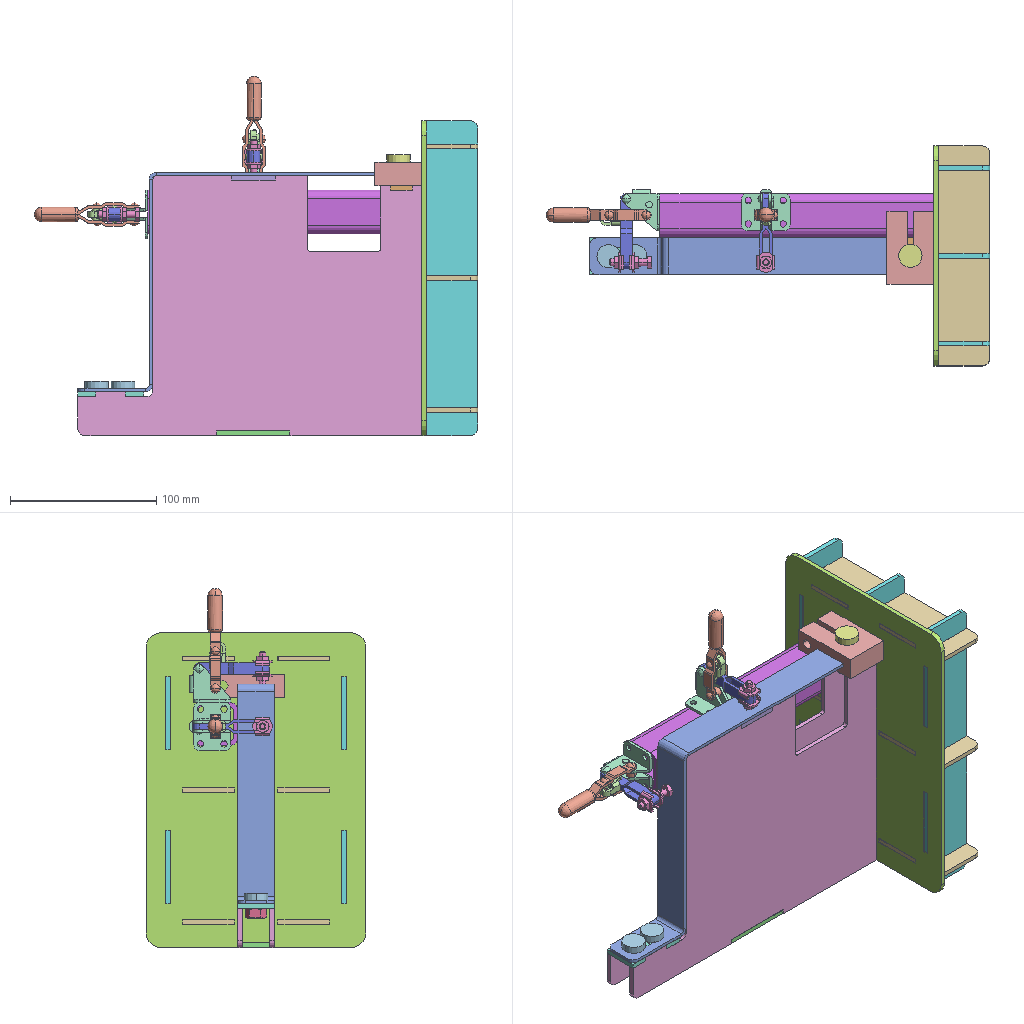Assembly | SolidWorks | 15 different items | 24 placed | box 303 x 150 x 245 mm
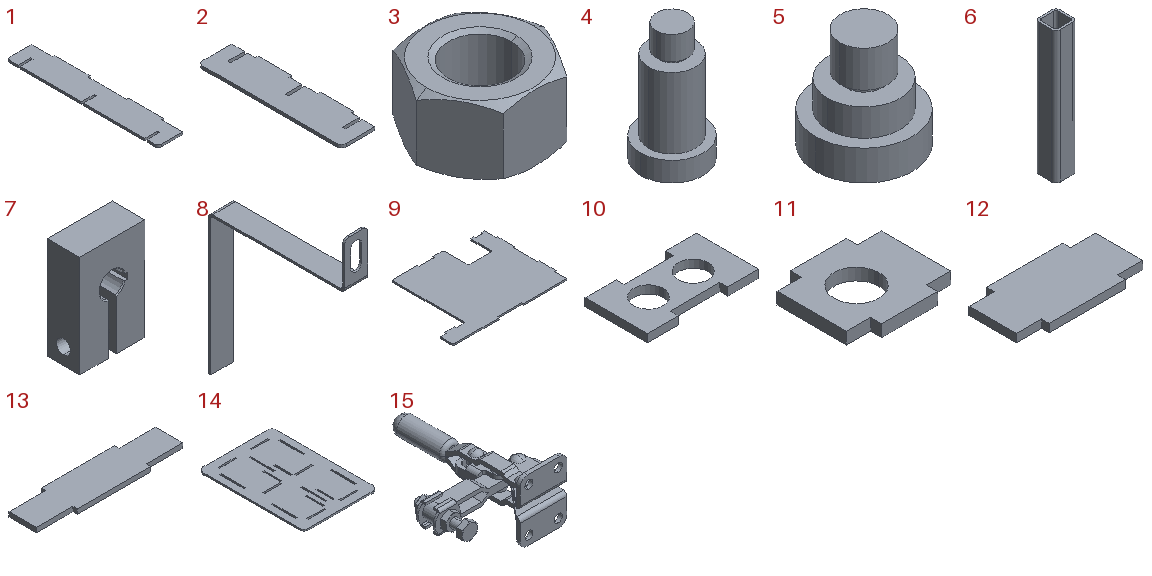Parts list (item | quantity | size | volume | features):
1 | x3 | 38 x 215 x 3.2 mm | 24453 mm3 | features FlatPattern 1, SMBaseFlange 1, SheetMetal 1
2 | x3 | 38 x 150 x 3.2 mm | 16900 mm3 | features FlatPattern 1, SMBaseFlange 1, SheetMetal 1
3 | x3 | 27.713 x 24 x 14.8 mm | 5071 mm3 | features RevCut 2, Chamfer 1, Extrusion 1, LPattern 1
4 | x1 | 16 x 16 x 30 mm | 3371 mm3 | features Revolution 1
5 | x2 | 16 x 16 x 16.5 mm | 1844 mm3 | features Revolution 1
6 | x1 | 30 x 30 x 187 mm | 56254 mm3 | features Attribute 1, Extrusion 1
7 | x1 | 32 x 16 x 50 mm | 20733 mm3 | features Chamfer 2, ICE 2, FlatPattern 1, HoleWzd 1, SMBaseFlange 1, SheetMetal 1
8 | x1 | 25 x 150 x 203 mm | 19203 mm3 | features Fillet 1, FlatPattern 1, ICE 1, SMBaseFlange 1, SheetMetal 1
9 | x2 | 238 x 177.7 x 3.2 mm | 99826 mm3 | features FlatPattern 1, SMBaseFlange 1, SheetMetal 1
10 | x1 | 45 x 25 x 3.2 mm | 2467 mm3 | features FlatPattern 1, SMBaseFlange 1, SheetMetal 1
11 | x1 | 28 x 24.6 x 3.2 mm | 1593 mm3 | features FlatPattern 1, SMBaseFlange 1, SheetMetal 1
12 | x1 | 50 x 24.6 x 3.2 mm | 3552 mm3 | features FlatPattern 1, SMBaseFlange 1, SheetMetal 1
13 | x1 | 100 x 24.6 x 3.2 mm | 6912 mm3 | features FlatPattern 1, SMBaseFlange 1, SheetMetal 1
14 | x1 | 150 x 215 x 3.2 mm | 96275 mm3 | features FlatPattern 1, SMBaseFlange 1, SheetMetal 1
15 | x2 | 56.45 x 77.62 x 33.3 mm | 10418 mm3 | features BaseBody 5
Mates (type | each side: item.copy, entity, surface, feature):
Coincident | 7.1 face plane Base-Flange1 | 8.1 face plane Base-Flange1
DistanceDim | 7.1 face plane Base-Flange1 | 8.1 face plane Base-Flange1 | 2 times
InPlace | 7.1 face plane Base-Flange1 | 14.1 plane
InPlace | 8.1 face plane Base-Flange1 | 9.1 plane
InPlace | 9.2 face plane Base-Flange1 | 10.1 plane
InPlace | 9.1 face plane Base-Flange1 | 11.1 plane
InPlace | 9.1 face plane Base-Flange1 | 12.1 plane
InPlace | 9.2 face plane Base-Flange1 | 13.1 plane
Concentric | 10.1 face cylinder Base-Flange1 | 3.1 face cone EndChamfer
Coincident | 10.1 face plane Base-Flange1 | 3.1 face plane BaseNut
Concentric | 10.1 face cylinder Base-Flange1 | 3.2 face cone EndChamfer
Coincident | 10.1 face plane Base-Flange1 | 3.2 face plane BaseNut
Concentric | 11.1 face cylinder Base-Flange1 | 3.3 face cone EndChamfer
Coincident | 11.1 face plane Base-Flange1 | 3.3 face plane BaseNut
Concentric | 10.1 face cylinder Base-Flange1 | 5.1 face cylinder Revolve1
Coincident | 8.1 face plane Base-Flange1 | 5.1 face plane Revolve1
Concentric | 7.1 face cylinder Base-Flange1 | 4.1 face cylinder Revolve1
Coincident | 7.1 face plane Base-Flange1 | 4.1 face plane Revolve1
Coincident | 14.1 face plane Base-Flange1 | 6.1 face plane Boss-Extrude1
DistanceDim | 6.1 face plane Boss-Extrude1 | 8.1 face plane Base-Flange1
Coincident | 9.2 face plane Base-Flange1 | 6.1 face plane Boss-Extrude1
Coincident | 6.1 face plane Boss-Extrude1 | 15.1 face plane TC1-1 vertical flange-base quick clamp [TCS1-1].step-1/_TCS1-1(seat).step-1-solid1 | 3 times
Coincident | 6.1 face plane Boss-Extrude1 | 15.2 face plane TC1-1 vertical flange-base quick clamp [TCS1-1].step-1/_TCS1-1(seat).step-1-solid1 | 2 times
DistanceDim | 15.2 face plane TC1-1 vertical flange-base quick clamp [TCS1-1].step-1/_TCS1-1(seat).step-1-solid1 | 9.2 face plane Base-Flange1
InPlace | 1.1 plane | assembly plane
InPlace | 2.1 plane | assembly plane